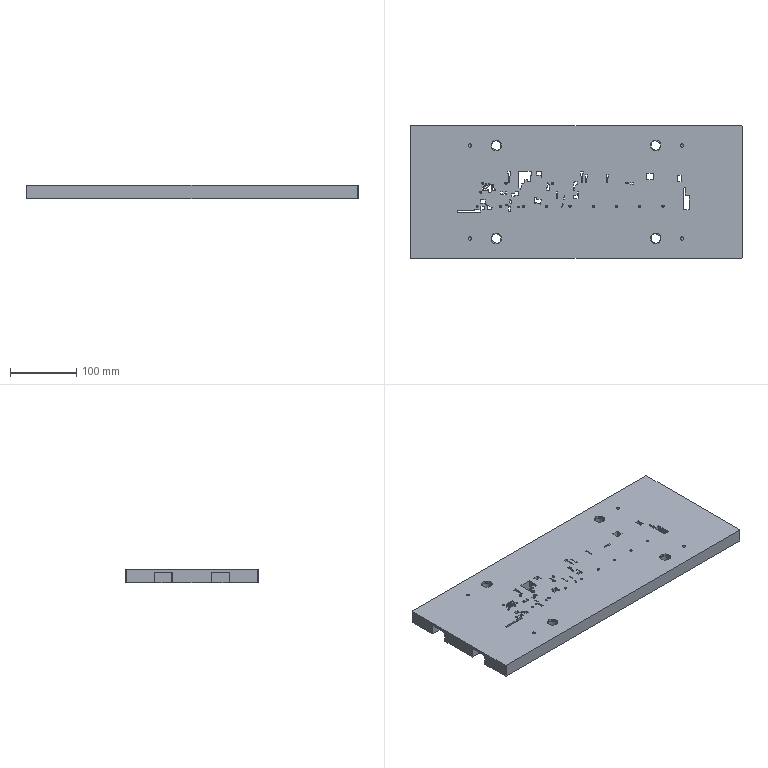Part | NX | features BREP 1 | 1 solid | 449 faces | box 500 x 200 x 20 mm | volume 1824471 mm3 | plane 272 | cylinder 173 | cone 4 | commonest cylinder face diameters 1.1 x69 0.9 x46 2 x10 2.5 x10 3.5 x10 3 x4